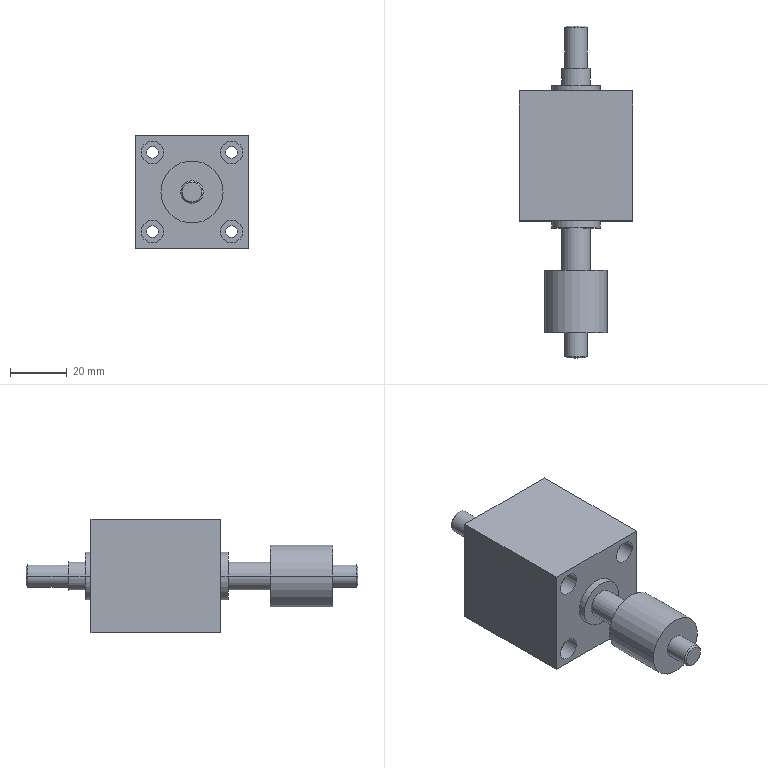Part | NX | 1 solid | 63 faces | box 40 x 117.5 x 40 mm | volume 81683 mm3 | cylinder 38 | plane 21 | cone 4 | commonest cylinder face diameters 8 x20 4.2 x8 10 x4 17 x4 22 x2